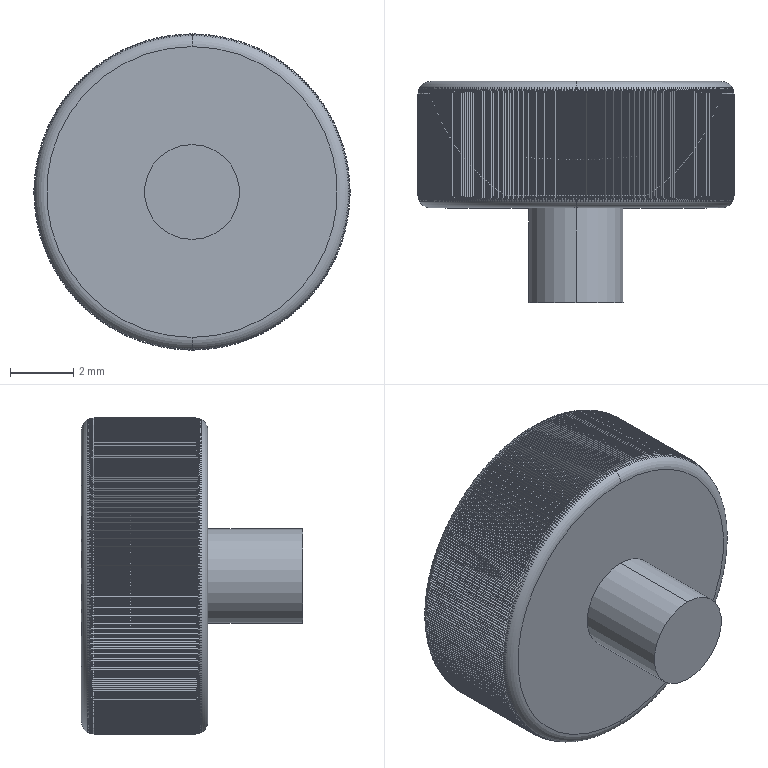Part | SolidWorks | features ICE 2, CirPattern 1, Extrusion 1, Fillet 1 | 1 solid | 1089 faces | box 10 x 7 x 10 mm | volume 331.248 mm3 | plane 723 | cylinder 362 | torus 4 | commonest cylinder face diameters 10 x360 3 x2